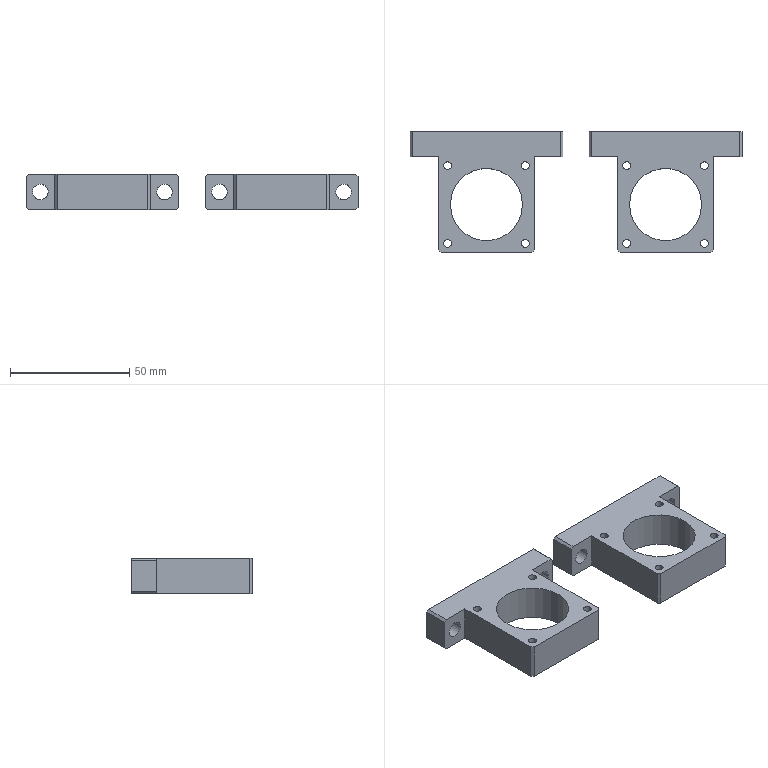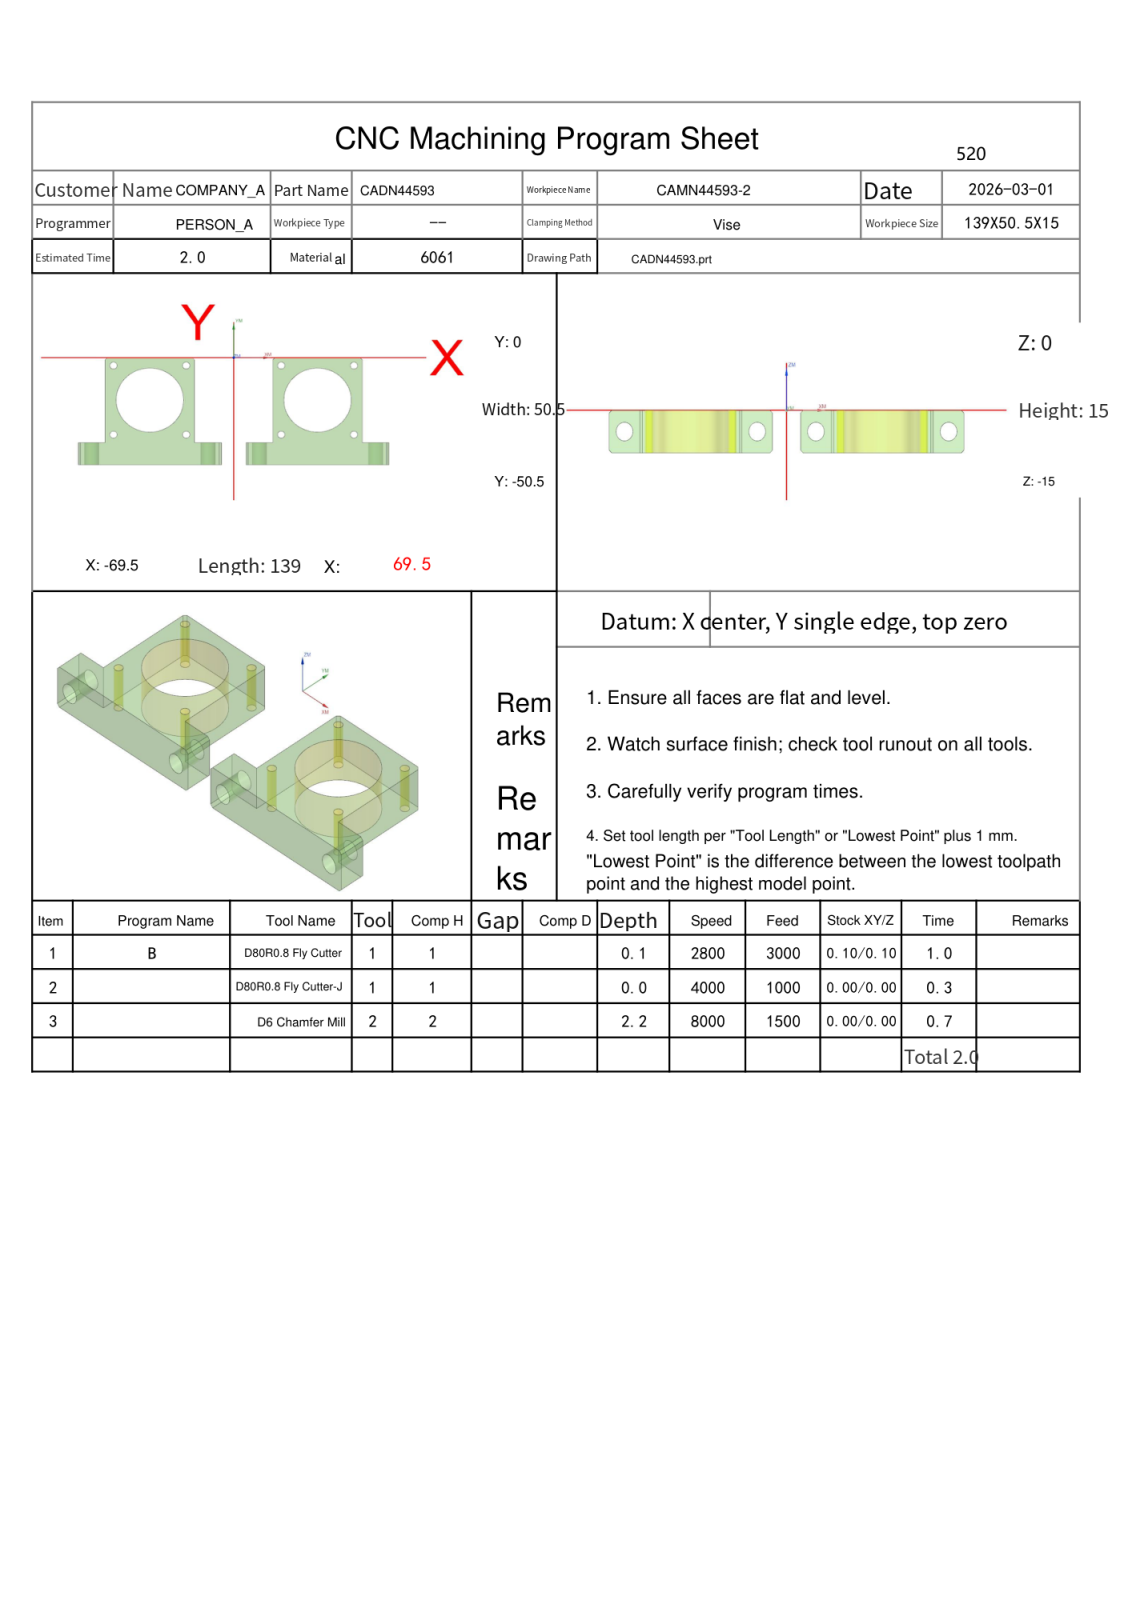NC program | NX | posted by the shop | part box 139 x 50.5 x 15 mm
Whole program:
%
O0001
(Machine time: 2.45 MIN)
(===Total Tool:2===)
(T1=D80R0.8 Fly Cutter D=80.  R=0.8  D-  H01 Z=0.    )
(T2=D6 Chamfer Mill   D=6.   R=0.   D-  H02 Z=-2.2  )
G80 G90 G17 G49 G40
G91 G28 Z0
M01
N1 T01 M06
(D80R0.8 Fly Cutter  D=80. R=0.8 H=01 ce=0.10 di=0.10)
G00 G90 G54 X121.597 Y-25.25 M03 S2800
G43 H01 Z50.
M08
Z6.011
G01 Z4.011 F3000.
X109.597
X-109.597
X-121.597
Z6.011
G00 X121.597
Z5.522
G01 Z3.522
X109.597
X-109.597
X-121.597
Z5.522
G00 X121.597
Z5.033
G01 Z3.033
X109.597
X-109.597
X-121.597
Z5.033
G00 X121.597
Z4.544
G01 Z2.544
X109.597
X-109.597
X-121.597
Z4.544
G00 Z50.
X121.597
Z4.056
G01 Z2.056
X109.597
X-109.597
X-121.597
Z4.056
G00 Z50.
X121.597
Z3.567
G01 Z1.567
X109.597
X-109.597
X-121.597
Z3.567
G00 Z50.
X121.597
Z3.078
G01 Z1.078
X109.597
X-109.597
X-121.597
Z3.078
G00 Z50.
X121.597
Z2.589
G01 Z.589
X109.597
X-109.597
X-121.597
Z2.589
G00 Z50.
X121.597
Z2.1
G01 Z.1
X109.597
X-109.597
X-121.597
Z2.1
G00 Z50.
G91 G28 Z0.0
M05
M09
G91 G28 Z0.0
M01
N2 T01 M06
(D80R0.8 Fly Cutter-J  D=80. R=0.8 H=01 ce=0.00 di=0.00)
G00 G90 G54 X121.499 Y-25.25 M03 S4000
G43 H01 Z50.
M08
Z2.
G01 Z0.0 F1000.
X109.499
X-109.499
X-121.499
Z2.
G00 Z50.
G91 G28 Z0.0
M05
M09
G91 G28 Z0.0
M01
N3 T02 M06
(D6 Chamfer Mill  D=6. R=0. H=02 ce=0.00 di=0.00)
G00 G90 G54 X-53.763 Y-3.737 M03 S8000
G43 H02 Z50.
M08
G98 G81 X-53.763 Y-3.737 Z-2.2 R3. F1000.
Y-36.263
X-21.237
Y-3.737
X21.237
X53.763
Y-36.263
X21.237
G80
G00 Z50.
G00 G90 X5.708 Y-39.01 M03 S6500
Z50.
Z.13
G01 Z-1.2 F1500.
G03 X6.048 Y-39.085 I.601 J1.907
G01 X6.102 Y-39.095
X6.151 Y-39.072
X6.241 Y-39.034
X6.5 Y-39.
X16.5
Y-1.
X16.534 Y-.741
X16.634 Y-.5
X16.793 Y-.293
X17.793 Y.707
X18. Y.866
X18.241 Y.966
X18.5 Y1.
X56.5
X56.759 Y.966
X57. Y.866
X57.207 Y.707
X58.207 Y-.293
X58.366 Y-.5
X58.466 Y-.741
X58.5 Y-1.
Y-39.
X68.5
X68.759 Y-39.034
X68.849 Y-39.072
X68.898 Y-39.095
X68.952 Y-39.085
G03 X69.292 Y-39.01 I-.261 J1.983
G01 Z.13
G00 Z10.
Y-51.49
Z.13
G01 Z-1.2
G03 X68.952 Y-51.415 I-.601 J-1.907
G01 X68.898 Y-51.405
X68.849 Y-51.428
X68.759 Y-51.466
X68.5 Y-51.5
X37.5
X6.5
X6.241 Y-51.466
X6.151 Y-51.428
X6.102 Y-51.405
X6.048 Y-51.415
G03 X5.708 Y-51.49 I.261 J-1.983
G01 Z.13
G00 Z10.
X21.73 Y-36.683
Z.405
G01 Z-1.2
G03 X21.878 Y-36.367 I-1.732 J1.
G01 X21.899 Y-36.316
X21.887 Y-36.263
G03 X21.237 Y-35.613 I-.65 J0.0
X20.587 Y-36.263 I0.0 J-.65
X21.237 Y-36.913 I.65 J0.0
X21.887 Y-36.263 I0.0 J.65
G01 X21.899 Y-36.21
X21.878 Y-36.16
G03 X21.73 Y-35.844 I-1.879 J-.684
G01 Z.405
G00 Z10.
X51.388 Y-20.394
Z.194
G01 Z-1.2
G03 X51.577 Y-20.101 I-1.579 J1.227
G01 X51.605 Y-20.054
X51.6 Y-20.
G03 X37.5 Y-5.9 I-14.1 J0.0
X23.4 Y-20. I0.0 J-14.1
X37.5 Y-34.1 I14.1 J0.0
X51.6 Y-20. I0.0 J14.1
G01 X51.605 Y-19.946
X51.577 Y-19.899
G03 X51.388 Y-19.606 I-1.768 J-.935
G01 Z.194
G00 Z10.
X21.73 Y-4.156
Z.405
G01 Z-1.2
G03 X21.878 Y-3.84 I-1.732 J1.
G01 X21.899 Y-3.79
X21.887 Y-3.737
G03 X21.237 Y-3.087 I-.65 J0.0
X20.587 Y-3.737 I0.0 J-.65
X21.237 Y-4.387 I.65 J0.0
X21.887 Y-3.737 I0.0 J.65
G01 X21.899 Y-3.684
X21.878 Y-3.633
G03 X21.73 Y-3.317 I-1.879 J-.684
G01 Z.405
G00 Z10.
X54.257 Y-4.156
Z.405
G01 Z-1.2
G03 X54.404 Y-3.84 I-1.732 J1.
G01 X54.426 Y-3.79
X54.413 Y-3.737
G03 X53.763 Y-3.087 I-.65 J0.0
X53.113 Y-3.737 I0.0 J-.65
X53.763 Y-4.387 I.65 J0.0
X54.413 Y-3.737 I0.0 J.65
G01 X54.426 Y-3.684
X54.404 Y-3.633
G03 X54.257 Y-3.317 I-1.879 J-.684
G01 Z.405
G00 Z10.
Y-36.683
Z.405
G01 Z-1.2
G03 X54.404 Y-36.367 I-1.732 J1.
G01 X54.426 Y-36.316
X54.413 Y-36.263
G03 X53.763 Y-35.613 I-.65 J0.0
X53.113 Y-36.263 I0.0 J-.65
X53.763 Y-36.913 I.65 J0.0
X54.413 Y-36.263 I0.0 J.65
G01 X54.426 Y-36.21
X54.404 Y-36.16
G03 X54.257 Y-35.844 I-1.879 J-.684
G01 Z.405
G00 Z10.
X-69.292 Y-39.01
Z.13
G01 Z-1.2
G03 X-68.952 Y-39.085 I.601 J1.907
G01 X-68.898 Y-39.095
X-68.849 Y-39.072
X-68.759 Y-39.034
X-68.5 Y-39.
X-58.5
Y-1.
X-58.466 Y-.741
X-58.366 Y-.5
X-58.207 Y-.293
X-57.207 Y.707
X-57. Y.866
X-56.759 Y.966
X-56.5 Y1.
X-18.5
X-18.241 Y.966
X-18. Y.866
X-17.793 Y.707
X-16.793 Y-.293
X-16.634 Y-.5
X-16.534 Y-.741
X-16.5 Y-1.
Y-39.
X-6.5
X-6.241 Y-39.034
X-6.151 Y-39.072
X-6.102 Y-39.095
X-6.048 Y-39.085
G03 X-5.708 Y-39.01 I-.261 J1.983
G01 Z.13
G00 Z10.
Y-51.49
Z.13
G01 Z-1.2
G03 X-6.048 Y-51.415 I-.601 J-1.907
G01 X-6.102 Y-51.405
X-6.151 Y-51.428
X-6.241 Y-51.466
X-6.5 Y-51.5
X-37.5
X-68.5
X-68.759 Y-51.466
X-68.849 Y-51.428
X-68.898 Y-51.405
X-68.952 Y-51.415
G03 X-69.292 Y-51.49 I.261 J-1.983
G01 Z.13
G00 Z10.
X-53.27 Y-36.683
Z.405
G01 Z-1.2
G03 X-53.122 Y-36.367 I-1.732 J1.
G01 X-53.101 Y-36.316
X-53.113 Y-36.263
G03 X-53.763 Y-35.613 I-.65 J0.0
X-54.413 Y-36.263 I0.0 J-.65
X-53.763 Y-36.913 I.65 J0.0
X-53.113 Y-36.263 I0.0 J.65
G01 X-53.101 Y-36.21
X-53.122 Y-36.16
G03 X-53.27 Y-35.844 I-1.879 J-.684
G01 Z.405
G00 Z10.
X-20.743 Y-36.683
Z.405
G01 Z-1.2
G03 X-20.596 Y-36.367 I-1.732 J1.
G01 X-20.574 Y-36.316
X-20.587 Y-36.263
G03 X-21.237 Y-35.613 I-.65 J0.0
X-21.887 Y-36.263 I0.0 J-.65
X-21.237 Y-36.913 I.65 J0.0
X-20.587 Y-36.263 I0.0 J.65
G01 X-20.574 Y-36.21
X-20.596 Y-36.16
G03 X-20.743 Y-35.844 I-1.879 J-.684
G01 Z.405
G00 Z10.
Y-4.156
Z.405
G01 Z-1.2
G03 X-20.596 Y-3.84 I-1.732 J1.
G01 X-20.574 Y-3.79
X-20.587 Y-3.737
G03 X-21.237 Y-3.087 I-.65 J0.0
X-21.887 Y-3.737 I0.0 J-.65
X-21.237 Y-4.387 I.65 J0.0
X-20.587 Y-3.737 I0.0 J.65
G01 X-20.574 Y-3.684
X-20.596 Y-3.633
G03 X-20.743 Y-3.317 I-1.879 J-.684
G01 Z.405
G00 Z10.
X-23.612 Y-20.394
Z.194
G01 Z-1.2
G03 X-23.423 Y-20.101 I-1.579 J1.227
G01 X-23.395 Y-20.054
X-23.4 Y-20.
G03 X-37.5 Y-5.9 I-14.1 J0.0
X-51.6 Y-20. I0.0 J-14.1
X-37.5 Y-34.1 I14.1 J0.0
X-23.4 Y-20. I0.0 J14.1
G01 X-23.395 Y-19.946
X-23.423 Y-19.899
G03 X-23.612 Y-19.606 I-1.768 J-.935
G01 Z.194
G00 Z10.
X-53.27 Y-4.156
Z.405
G01 Z-1.2
G03 X-53.122 Y-3.84 I-1.732 J1.
G01 X-53.101 Y-3.79
X-53.113 Y-3.737
G03 X-53.763 Y-3.087 I-.65 J0.0
X-54.413 Y-3.737 I0.0 J-.65
X-53.763 Y-4.387 I.65 J0.0
X-53.113 Y-3.737 I0.0 J.65
G01 X-53.101 Y-3.684
X-53.122 Y-3.633
G03 X-53.27 Y-3.317 I-1.879 J-.684
G01 Z.405
G00 Z50.
G00 G90 X70.208 Y-37.1 M03 S6500
Z50.
Z-.2
G01 Z-1.7 F1500.
X70.199 Y-37.168
X70.2 Y-37.237
Y-53.263
X70.199 Y-53.332
X70.208 Y-53.4
Z-.2
G00 Z50.
X4.792
Z-.2
G01 Z-1.7
X4.801 Y-53.332
X4.8 Y-53.263
Y-37.237
X4.801 Y-37.168
X4.792 Y-37.1
Z-.2
G00 X-4.792
G01 Z-1.7
X-4.801 Y-37.168
X-4.8 Y-37.237
Y-53.263
X-4.801 Y-53.332
X-4.792 Y-53.4
Z-.2
G00 Z50.
X-70.208
Z-.2
G01 Z-1.7
X-70.199 Y-53.332
X-70.2 Y-53.263
Y-37.237
X-70.199 Y-37.168
X-70.208 Y-37.1
Z-.2
G00 Z50.
M05
M09
G91 G28 Z0.0
G91 G28 Y0.0
M30
%